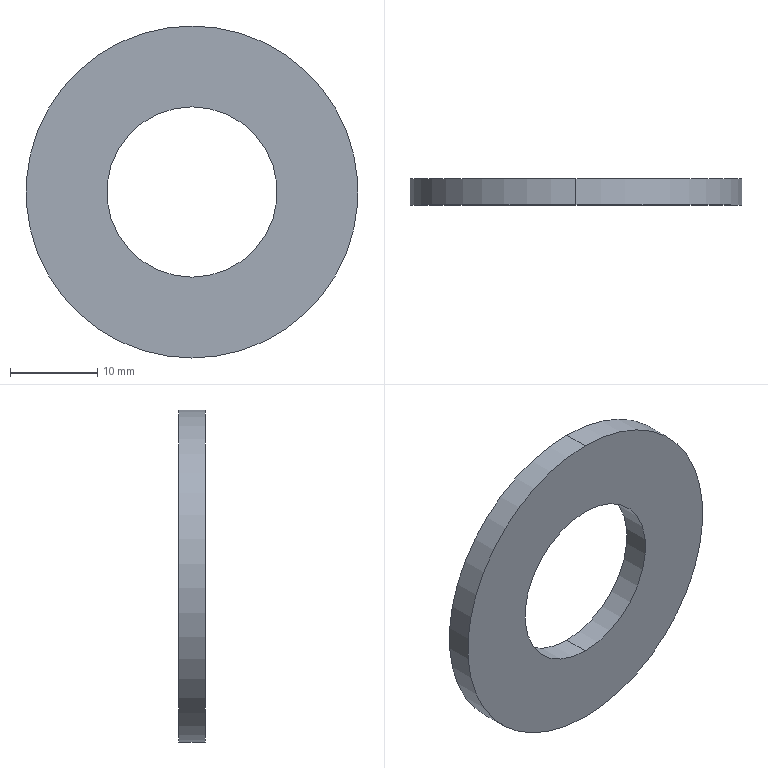Part | NX | features BREP 1 | 1 solid | 6 faces | box 38 x 3 x 38 mm | volume 2506 mm3 | cylinder 4 | plane 2 | commonest cylinder face diameters 19.5 x2 38 x2
STEP:
#1=CARTESIAN_POINT('',(67.55,263.017,-47.85));
#2=VERTEX_POINT('',#1);
#3=CARTESIAN_POINT('',(67.55,263.017,-28.35));
#4=VERTEX_POINT('',#3);
#5=CARTESIAN_POINT('',(67.55,263.017,-38.1));
#6=DIRECTION('',(0.,1.,0.));
#7=DIRECTION('',(0.,0.,1.));
#8=AXIS2_PLACEMENT_3D('',#5,#6,#7);
#9=CIRCLE('',#8,9.75);
#10=EDGE_CURVE('',#2,#4,#9,.T.);
#11=ORIENTED_EDGE('',*,*,#10,.F.);
#12=CARTESIAN_POINT('',(67.55,266.017,-47.85));
#13=VERTEX_POINT('',#12);
#14=CARTESIAN_POINT('',(67.55,266.017,-47.85));
#15=DIRECTION('',(0.,1.,0.));
#16=VECTOR('',#15,1000.);
#17=LINE('',#14,#16);
#18=EDGE_CURVE('',#2,#13,#17,.T.);
#19=ORIENTED_EDGE('',*,*,#18,.T.);
#20=CARTESIAN_POINT('',(67.55,266.017,-28.35));
#21=VERTEX_POINT('',#20);
#22=CARTESIAN_POINT('',(67.55,266.017,-38.1));
#23=DIRECTION('',(0.,1.,0.));
#24=DIRECTION('',(0.,0.,1.));
#25=AXIS2_PLACEMENT_3D('',#22,#23,#24);
#26=CIRCLE('',#25,9.75);
#27=EDGE_CURVE('',#13,#21,#26,.T.);
#28=ORIENTED_EDGE('',*,*,#27,.T.);
#29=CARTESIAN_POINT('',(67.55,266.017,-28.35));
#30=DIRECTION('',(0.,1.,0.));
#31=VECTOR('',#30,1000.);
#32=LINE('',#29,#31);
#33=EDGE_CURVE('',#4,#21,#32,.T.);
#34=ORIENTED_EDGE('',*,*,#33,.F.);
#35=EDGE_LOOP('',(#11,#19,#28,#34));
#36=FACE_BOUND('',#35,.T.);
#37=CARTESIAN_POINT('',(67.55,266.017,-38.1));
#38=DIRECTION('',(0.,1.,0.));
#39=DIRECTION('',(0.,0.,-1.));
#40=AXIS2_PLACEMENT_3D('',#37,#38,#39);
#41=CYLINDRICAL_SURFACE('',#40,9.75);
#42=ADVANCED_FACE('',(#36),#41,.F.);
#43=CARTESIAN_POINT('',(67.55,263.017,-19.1));
#44=VERTEX_POINT('',#43);
#45=CARTESIAN_POINT('',(67.55,263.017,-57.1));
#46=VERTEX_POINT('',#45);
#47=CARTESIAN_POINT('',(67.55,263.017,-38.1));
#48=DIRECTION('',(0.,1.,0.));
#49=DIRECTION('',(0.,0.,1.));
#50=AXIS2_PLACEMENT_3D('',#47,#48,#49);
#51=CIRCLE('',#50,19.);
#52=EDGE_CURVE('',#44,#46,#51,.T.);
#53=ORIENTED_EDGE('',*,*,#52,.T.);
#54=CARTESIAN_POINT('',(67.55,266.017,-57.1));
#55=VERTEX_POINT('',#54);
#56=CARTESIAN_POINT('',(67.55,266.017,-57.1));
#57=DIRECTION('',(0.,1.,0.));
#58=VECTOR('',#57,1000.);
#59=LINE('',#56,#58);
#60=EDGE_CURVE('',#46,#55,#59,.T.);
#61=ORIENTED_EDGE('',*,*,#60,.T.);
#62=CARTESIAN_POINT('',(67.55,266.017,-19.1));
#63=VERTEX_POINT('',#62);
#64=CARTESIAN_POINT('',(67.55,266.017,-38.1));
#65=DIRECTION('',(0.,1.,0.));
#66=DIRECTION('',(0.,0.,1.));
#67=AXIS2_PLACEMENT_3D('',#64,#65,#66);
#68=CIRCLE('',#67,19.);
#69=EDGE_CURVE('',#63,#55,#68,.T.);
#70=ORIENTED_EDGE('',*,*,#69,.F.);
#71=CARTESIAN_POINT('',(67.55,266.017,-19.1));
#72=DIRECTION('',(0.,1.,0.));
#73=VECTOR('',#72,1000.);
#74=LINE('',#71,#73);
#75=EDGE_CURVE('',#44,#63,#74,.T.);
#76=ORIENTED_EDGE('',*,*,#75,.F.);
#77=EDGE_LOOP('',(#53,#61,#70,#76));
#78=FACE_BOUND('',#77,.T.);
#79=CARTESIAN_POINT('',(67.55,266.017,-38.1));
#80=DIRECTION('',(0.,1.,0.));
#81=DIRECTION('',(0.,0.,-1.));
#82=AXIS2_PLACEMENT_3D('',#79,#80,#81);
#83=CYLINDRICAL_SURFACE('',#82,19.);
#84=ADVANCED_FACE('',(#78),#83,.T.);
#85=ORIENTED_EDGE('',*,*,#60,.F.);
#86=CARTESIAN_POINT('',(67.55,263.017,-38.1));
#87=DIRECTION('',(0.,1.,0.));
#88=DIRECTION('',(0.,0.,1.));
#89=AXIS2_PLACEMENT_3D('',#86,#87,#88);
#90=CIRCLE('',#89,19.);
#91=EDGE_CURVE('',#46,#44,#90,.T.);
#92=ORIENTED_EDGE('',*,*,#91,.T.);
#93=ORIENTED_EDGE('',*,*,#75,.T.);
#94=CARTESIAN_POINT('',(67.55,266.017,-38.1));
#95=DIRECTION('',(0.,1.,0.));
#96=DIRECTION('',(0.,0.,1.));
#97=AXIS2_PLACEMENT_3D('',#94,#95,#96);
#98=CIRCLE('',#97,19.);
#99=EDGE_CURVE('',#55,#63,#98,.T.);
#100=ORIENTED_EDGE('',*,*,#99,.F.);
#101=EDGE_LOOP('',(#85,#92,#93,#100));
#102=FACE_BOUND('',#101,.T.);
#103=CARTESIAN_POINT('',(67.55,266.017,-38.1));
#104=DIRECTION('',(0.,1.,0.));
#105=DIRECTION('',(0.,0.,-1.));
#106=AXIS2_PLACEMENT_3D('',#103,#104,#105);
#107=CYLINDRICAL_SURFACE('',#106,19.);
#108=ADVANCED_FACE('',(#102),#107,.T.);
#109=CARTESIAN_POINT('',(67.55,266.017,-38.1));
#110=DIRECTION('',(0.,1.,0.));
#111=DIRECTION('',(0.,0.,1.));
#112=AXIS2_PLACEMENT_3D('',#109,#110,#111);
#113=CIRCLE('',#112,9.75);
#114=EDGE_CURVE('',#21,#13,#113,.T.);
#115=ORIENTED_EDGE('',*,*,#114,.F.);
#116=ORIENTED_EDGE('',*,*,#27,.F.);
#117=EDGE_LOOP('',(#115,#116));
#118=FACE_BOUND('',#117,.T.);
#119=ORIENTED_EDGE('',*,*,#69,.T.);
#120=ORIENTED_EDGE('',*,*,#99,.T.);
#121=EDGE_LOOP('',(#119,#120));
#122=FACE_BOUND('',#121,.T.);
#123=CARTESIAN_POINT('',(86.55,266.017,-38.1));
#124=DIRECTION('',(0.,-1.,0.));
#125=DIRECTION('',(0.,0.,1.));
#126=AXIS2_PLACEMENT_3D('',#123,#124,#125);
#127=PLANE('',#126);
#128=ADVANCED_FACE('',(#118,#122),#127,.F.);
#129=ORIENTED_EDGE('',*,*,#18,.F.);
#130=CARTESIAN_POINT('',(67.55,263.017,-38.1));
#131=DIRECTION('',(0.,1.,0.));
#132=DIRECTION('',(0.,0.,1.));
#133=AXIS2_PLACEMENT_3D('',#130,#131,#132);
#134=CIRCLE('',#133,9.75);
#135=EDGE_CURVE('',#4,#2,#134,.T.);
#136=ORIENTED_EDGE('',*,*,#135,.F.);
#137=ORIENTED_EDGE('',*,*,#33,.T.);
#138=ORIENTED_EDGE('',*,*,#114,.T.);
#139=EDGE_LOOP('',(#129,#136,#137,#138));
#140=FACE_BOUND('',#139,.T.);
#141=CARTESIAN_POINT('',(67.55,266.017,-38.1));
#142=DIRECTION('',(0.,1.,0.));
#143=DIRECTION('',(0.,0.,-1.));
#144=AXIS2_PLACEMENT_3D('',#141,#142,#143);
#145=CYLINDRICAL_SURFACE('',#144,9.75);
#146=ADVANCED_FACE('',(#140),#145,.F.);
#147=ORIENTED_EDGE('',*,*,#52,.F.);
#148=ORIENTED_EDGE('',*,*,#91,.F.);
#149=EDGE_LOOP('',(#147,#148));
#150=FACE_BOUND('',#149,.T.);
#151=ORIENTED_EDGE('',*,*,#135,.T.);
#152=ORIENTED_EDGE('',*,*,#10,.T.);
#153=EDGE_LOOP('',(#151,#152));
#154=FACE_BOUND('',#153,.T.);
#155=CARTESIAN_POINT('',(77.3,263.017,-38.1));
#156=DIRECTION('',(0.,1.,0.));
#157=DIRECTION('',(0.,0.,-1.));
#158=AXIS2_PLACEMENT_3D('',#155,#156,#157);
#159=PLANE('',#158);
#160=ADVANCED_FACE('',(#150,#154),#159,.F.);
#161=CLOSED_SHELL('',(#42,#84,#108,#128,#146,#160));
#162=MANIFOLD_SOLID_BREP('',#161);
#163=(LENGTH_UNIT()NAMED_UNIT(*)SI_UNIT(.MILLI.,.METRE.));
#164=UNCERTAINTY_MEASURE_WITH_UNIT(LENGTH_MEASURE(0.00001),#163,'','');
#165=(NAMED_UNIT(*)PLANE_ANGLE_UNIT()SI_UNIT($,.RADIAN.));
#166=(NAMED_UNIT(*)SI_UNIT($,.STERADIAN.)SOLID_ANGLE_UNIT());
#167=(GEOMETRIC_REPRESENTATION_CONTEXT(3)GLOBAL_UNCERTAINTY_ASSIGNED_CONTEXT((#164))GLOBAL_UNIT_ASSIGNED_CONTEXT((#163,#165,#166))REPRESENTATION_CONTEXT('',''));
#168=ADVANCED_BREP_SHAPE_REPRESENTATION('',(#162),#167);